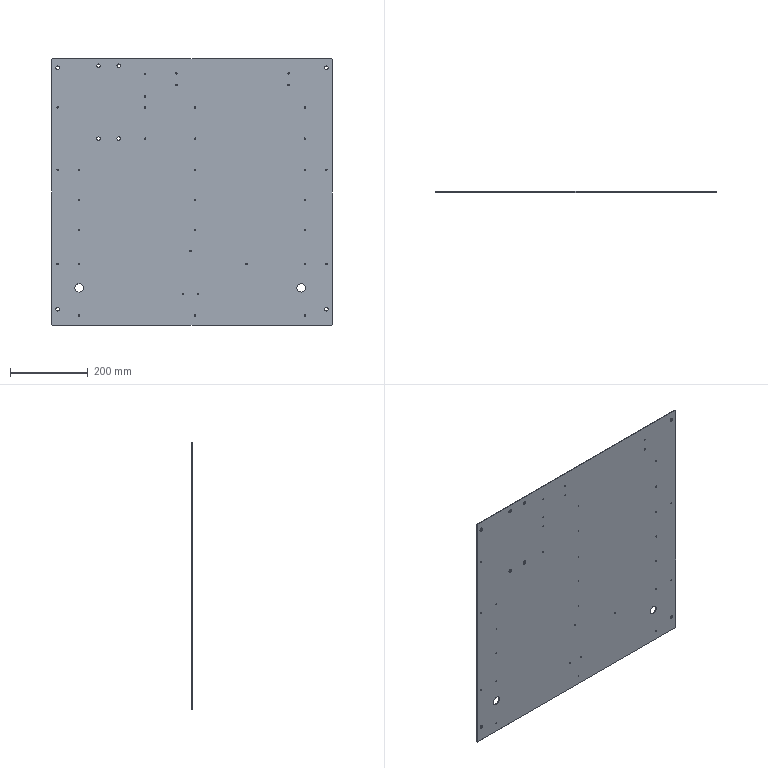Part | NX | features solid 2 | 1 solid | 100 faces | box 720 x 2.5 x 684 mm | volume 1227268 mm3 | cylinder 94 | plane 6 | commonest cylinder face diameters 3.242 x70 9 x8 9.2 x8 4 x4 22 x4